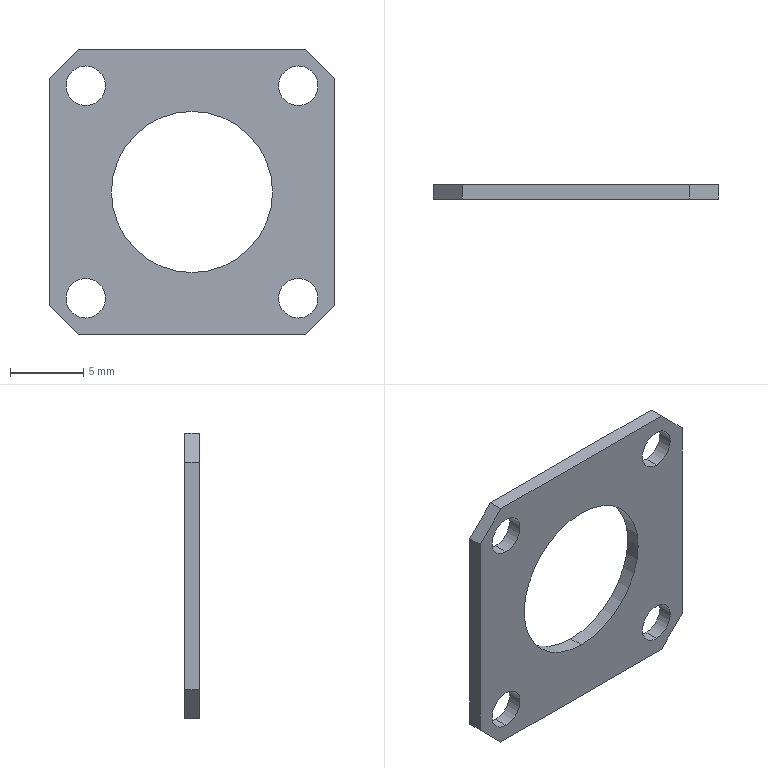Part | SolidWorks | features Extrusion 1, ICE 1 | 1 solid | 20 faces | box 19.5 x 1 x 19.5 mm | volume 254.315 mm3 | cylinder 10 | plane 10 | commonest cylinder face diameters 2.7 x8 11 x2
STEP:
#1=CARTESIAN_POINT('',(-7.25,0.,5.9));
#2=VERTEX_POINT('',#1);
#3=CARTESIAN_POINT('',(-7.25,0.,8.6));
#4=VERTEX_POINT('',#3);
#5=CARTESIAN_POINT('',(-7.25,0.,7.25));
#6=DIRECTION('',(0.,1.,0.));
#7=DIRECTION('',(0.,0.,1.));
#8=AXIS2_PLACEMENT_3D('',#5,#6,#7);
#9=CIRCLE('',#8,1.35);
#10=EDGE_CURVE('',#2,#4,#9,.T.);
#11=ORIENTED_EDGE('',*,*,#10,.F.);
#12=CARTESIAN_POINT('',(-7.25,1.,5.9));
#13=VERTEX_POINT('',#12);
#14=CARTESIAN_POINT('',(-7.25,0.,5.9));
#15=DIRECTION('',(0.,1.,0.));
#16=VECTOR('',#15,1000.);
#17=LINE('',#14,#16);
#18=EDGE_CURVE('',#2,#13,#17,.T.);
#19=ORIENTED_EDGE('',*,*,#18,.T.);
#20=CARTESIAN_POINT('',(-7.25,1.,8.6));
#21=VERTEX_POINT('',#20);
#22=CARTESIAN_POINT('',(-7.25,1.,7.25));
#23=DIRECTION('',(0.,1.,0.));
#24=DIRECTION('',(0.,0.,1.));
#25=AXIS2_PLACEMENT_3D('',#22,#23,#24);
#26=CIRCLE('',#25,1.35);
#27=EDGE_CURVE('',#13,#21,#26,.T.);
#28=ORIENTED_EDGE('',*,*,#27,.T.);
#29=CARTESIAN_POINT('',(-7.25,0.,8.6));
#30=DIRECTION('',(0.,1.,0.));
#31=VECTOR('',#30,1000.);
#32=LINE('',#29,#31);
#33=EDGE_CURVE('',#4,#21,#32,.T.);
#34=ORIENTED_EDGE('',*,*,#33,.F.);
#35=EDGE_LOOP('',(#11,#19,#28,#34));
#36=FACE_OUTER_BOUND('',#35,.T.);
#37=CARTESIAN_POINT('',(-7.25,0.,7.25));
#38=DIRECTION('',(0.,1.,0.));
#39=DIRECTION('',(0.,0.,1.));
#40=AXIS2_PLACEMENT_3D('',#37,#38,#39);
#41=CYLINDRICAL_SURFACE('',#40,1.35);
#42=ADVANCED_FACE('',(#36),#41,.F.);
#43=CARTESIAN_POINT('',(7.25,0.,5.9));
#44=VERTEX_POINT('',#43);
#45=CARTESIAN_POINT('',(7.25,0.,8.6));
#46=VERTEX_POINT('',#45);
#47=CARTESIAN_POINT('',(7.25,0.,7.25));
#48=DIRECTION('',(0.,1.,0.));
#49=DIRECTION('',(0.,0.,1.));
#50=AXIS2_PLACEMENT_3D('',#47,#48,#49);
#51=CIRCLE('',#50,1.35);
#52=EDGE_CURVE('',#44,#46,#51,.T.);
#53=ORIENTED_EDGE('',*,*,#52,.F.);
#54=CARTESIAN_POINT('',(7.25,1.,5.9));
#55=VERTEX_POINT('',#54);
#56=CARTESIAN_POINT('',(7.25,0.,5.9));
#57=DIRECTION('',(0.,1.,0.));
#58=VECTOR('',#57,1000.);
#59=LINE('',#56,#58);
#60=EDGE_CURVE('',#44,#55,#59,.T.);
#61=ORIENTED_EDGE('',*,*,#60,.T.);
#62=CARTESIAN_POINT('',(7.25,1.,8.6));
#63=VERTEX_POINT('',#62);
#64=CARTESIAN_POINT('',(7.25,1.,7.25));
#65=DIRECTION('',(0.,1.,0.));
#66=DIRECTION('',(0.,0.,1.));
#67=AXIS2_PLACEMENT_3D('',#64,#65,#66);
#68=CIRCLE('',#67,1.35);
#69=EDGE_CURVE('',#55,#63,#68,.T.);
#70=ORIENTED_EDGE('',*,*,#69,.T.);
#71=CARTESIAN_POINT('',(7.25,0.,8.6));
#72=DIRECTION('',(0.,1.,0.));
#73=VECTOR('',#72,1000.);
#74=LINE('',#71,#73);
#75=EDGE_CURVE('',#46,#63,#74,.T.);
#76=ORIENTED_EDGE('',*,*,#75,.F.);
#77=EDGE_LOOP('',(#53,#61,#70,#76));
#78=FACE_OUTER_BOUND('',#77,.T.);
#79=CARTESIAN_POINT('',(7.25,0.,7.25));
#80=DIRECTION('',(0.,1.,0.));
#81=DIRECTION('',(0.,0.,1.));
#82=AXIS2_PLACEMENT_3D('',#79,#80,#81);
#83=CYLINDRICAL_SURFACE('',#82,1.35);
#84=ADVANCED_FACE('',(#78),#83,.F.);
#85=CARTESIAN_POINT('',(7.25,0.,-8.6));
#86=VERTEX_POINT('',#85);
#87=CARTESIAN_POINT('',(7.25,0.,-5.9));
#88=VERTEX_POINT('',#87);
#89=CARTESIAN_POINT('',(7.25,0.,-7.25));
#90=DIRECTION('',(0.,1.,0.));
#91=DIRECTION('',(0.,0.,1.));
#92=AXIS2_PLACEMENT_3D('',#89,#90,#91);
#93=CIRCLE('',#92,1.35);
#94=EDGE_CURVE('',#86,#88,#93,.T.);
#95=ORIENTED_EDGE('',*,*,#94,.F.);
#96=CARTESIAN_POINT('',(7.25,1.,-8.6));
#97=VERTEX_POINT('',#96);
#98=CARTESIAN_POINT('',(7.25,0.,-8.6));
#99=DIRECTION('',(0.,1.,0.));
#100=VECTOR('',#99,1000.);
#101=LINE('',#98,#100);
#102=EDGE_CURVE('',#86,#97,#101,.T.);
#103=ORIENTED_EDGE('',*,*,#102,.T.);
#104=CARTESIAN_POINT('',(7.25,1.,-5.9));
#105=VERTEX_POINT('',#104);
#106=CARTESIAN_POINT('',(7.25,1.,-7.25));
#107=DIRECTION('',(0.,1.,0.));
#108=DIRECTION('',(0.,0.,1.));
#109=AXIS2_PLACEMENT_3D('',#106,#107,#108);
#110=CIRCLE('',#109,1.35);
#111=EDGE_CURVE('',#97,#105,#110,.T.);
#112=ORIENTED_EDGE('',*,*,#111,.T.);
#113=CARTESIAN_POINT('',(7.25,0.,-5.9));
#114=DIRECTION('',(0.,1.,0.));
#115=VECTOR('',#114,1000.);
#116=LINE('',#113,#115);
#117=EDGE_CURVE('',#88,#105,#116,.T.);
#118=ORIENTED_EDGE('',*,*,#117,.F.);
#119=EDGE_LOOP('',(#95,#103,#112,#118));
#120=FACE_OUTER_BOUND('',#119,.T.);
#121=CARTESIAN_POINT('',(7.25,0.,-7.25));
#122=DIRECTION('',(0.,1.,0.));
#123=DIRECTION('',(0.,0.,1.));
#124=AXIS2_PLACEMENT_3D('',#121,#122,#123);
#125=CYLINDRICAL_SURFACE('',#124,1.35);
#126=ADVANCED_FACE('',(#120),#125,.F.);
#127=CARTESIAN_POINT('',(-7.25,0.,-8.6));
#128=VERTEX_POINT('',#127);
#129=CARTESIAN_POINT('',(-7.25,0.,-5.9));
#130=VERTEX_POINT('',#129);
#131=CARTESIAN_POINT('',(-7.25,0.,-7.25));
#132=DIRECTION('',(0.,1.,0.));
#133=DIRECTION('',(0.,0.,1.));
#134=AXIS2_PLACEMENT_3D('',#131,#132,#133);
#135=CIRCLE('',#134,1.35);
#136=EDGE_CURVE('',#128,#130,#135,.T.);
#137=ORIENTED_EDGE('',*,*,#136,.F.);
#138=CARTESIAN_POINT('',(-7.25,1.,-8.6));
#139=VERTEX_POINT('',#138);
#140=CARTESIAN_POINT('',(-7.25,0.,-8.6));
#141=DIRECTION('',(0.,1.,0.));
#142=VECTOR('',#141,1000.);
#143=LINE('',#140,#142);
#144=EDGE_CURVE('',#128,#139,#143,.T.);
#145=ORIENTED_EDGE('',*,*,#144,.T.);
#146=CARTESIAN_POINT('',(-7.25,1.,-5.9));
#147=VERTEX_POINT('',#146);
#148=CARTESIAN_POINT('',(-7.25,1.,-7.25));
#149=DIRECTION('',(0.,1.,0.));
#150=DIRECTION('',(0.,0.,1.));
#151=AXIS2_PLACEMENT_3D('',#148,#149,#150);
#152=CIRCLE('',#151,1.35);
#153=EDGE_CURVE('',#139,#147,#152,.T.);
#154=ORIENTED_EDGE('',*,*,#153,.T.);
#155=CARTESIAN_POINT('',(-7.25,0.,-5.9));
#156=DIRECTION('',(0.,1.,0.));
#157=VECTOR('',#156,1000.);
#158=LINE('',#155,#157);
#159=EDGE_CURVE('',#130,#147,#158,.T.);
#160=ORIENTED_EDGE('',*,*,#159,.F.);
#161=EDGE_LOOP('',(#137,#145,#154,#160));
#162=FACE_OUTER_BOUND('',#161,.T.);
#163=CARTESIAN_POINT('',(-7.25,0.,-7.25));
#164=DIRECTION('',(0.,1.,0.));
#165=DIRECTION('',(0.,0.,1.));
#166=AXIS2_PLACEMENT_3D('',#163,#164,#165);
#167=CYLINDRICAL_SURFACE('',#166,1.35);
#168=ADVANCED_FACE('',(#162),#167,.F.);
#169=CARTESIAN_POINT('',(0.,1.,-5.5));
#170=VERTEX_POINT('',#169);
#171=CARTESIAN_POINT('',(0.,1.,5.5));
#172=VERTEX_POINT('',#171);
#173=CARTESIAN_POINT('',(0.,1.,0.));
#174=DIRECTION('',(0.,1.,0.));
#175=DIRECTION('',(0.,0.,1.));
#176=AXIS2_PLACEMENT_3D('',#173,#174,#175);
#177=CIRCLE('',#176,5.5);
#178=EDGE_CURVE('',#170,#172,#177,.T.);
#179=ORIENTED_EDGE('',*,*,#178,.T.);
#180=CARTESIAN_POINT('',(0.,0.,5.5));
#181=VERTEX_POINT('',#180);
#182=CARTESIAN_POINT('',(0.,1.,5.5));
#183=DIRECTION('',(0.,-1.,0.));
#184=VECTOR('',#183,1000.);
#185=LINE('',#182,#184);
#186=EDGE_CURVE('',#172,#181,#185,.T.);
#187=ORIENTED_EDGE('',*,*,#186,.T.);
#188=CARTESIAN_POINT('',(0.,0.,-5.5));
#189=VERTEX_POINT('',#188);
#190=CARTESIAN_POINT('',(0.,0.,0.));
#191=DIRECTION('',(0.,1.,0.));
#192=DIRECTION('',(0.,0.,1.));
#193=AXIS2_PLACEMENT_3D('',#190,#191,#192);
#194=CIRCLE('',#193,5.5);
#195=EDGE_CURVE('',#189,#181,#194,.T.);
#196=ORIENTED_EDGE('',*,*,#195,.F.);
#197=CARTESIAN_POINT('',(0.,1.,-5.5));
#198=DIRECTION('',(0.,-1.,0.));
#199=VECTOR('',#198,1000.);
#200=LINE('',#197,#199);
#201=EDGE_CURVE('',#170,#189,#200,.T.);
#202=ORIENTED_EDGE('',*,*,#201,.F.);
#203=EDGE_LOOP('',(#179,#187,#196,#202));
#204=FACE_OUTER_BOUND('',#203,.T.);
#205=CARTESIAN_POINT('',(0.,1.,0.));
#206=DIRECTION('',(0.,-1.,0.));
#207=DIRECTION('',(0.,0.,-1.));
#208=AXIS2_PLACEMENT_3D('',#205,#206,#207);
#209=CYLINDRICAL_SURFACE('',#208,5.5);
#210=ADVANCED_FACE('',(#204),#209,.F.);
#211=CARTESIAN_POINT('',(-7.25,1.,7.25));
#212=DIRECTION('',(0.,1.,0.));
#213=DIRECTION('',(0.,0.,1.));
#214=AXIS2_PLACEMENT_3D('',#211,#212,#213);
#215=CIRCLE('',#214,1.35);
#216=EDGE_CURVE('',#21,#13,#215,.T.);
#217=ORIENTED_EDGE('',*,*,#216,.F.);
#218=ORIENTED_EDGE('',*,*,#27,.F.);
#219=EDGE_LOOP('',(#217,#218));
#220=FACE_BOUND('',#219,.T.);
#221=CARTESIAN_POINT('',(7.25,1.,7.25));
#222=DIRECTION('',(0.,1.,0.));
#223=DIRECTION('',(0.,0.,1.));
#224=AXIS2_PLACEMENT_3D('',#221,#222,#223);
#225=CIRCLE('',#224,1.35);
#226=EDGE_CURVE('',#63,#55,#225,.T.);
#227=ORIENTED_EDGE('',*,*,#226,.F.);
#228=ORIENTED_EDGE('',*,*,#69,.F.);
#229=EDGE_LOOP('',(#227,#228));
#230=FACE_BOUND('',#229,.T.);
#231=CARTESIAN_POINT('',(7.25,1.,-7.25));
#232=DIRECTION('',(0.,1.,0.));
#233=DIRECTION('',(0.,0.,1.));
#234=AXIS2_PLACEMENT_3D('',#231,#232,#233);
#235=CIRCLE('',#234,1.35);
#236=EDGE_CURVE('',#105,#97,#235,.T.);
#237=ORIENTED_EDGE('',*,*,#236,.F.);
#238=ORIENTED_EDGE('',*,*,#111,.F.);
#239=EDGE_LOOP('',(#237,#238));
#240=FACE_BOUND('',#239,.T.);
#241=CARTESIAN_POINT('',(-7.25,1.,-7.25));
#242=DIRECTION('',(0.,1.,0.));
#243=DIRECTION('',(0.,0.,1.));
#244=AXIS2_PLACEMENT_3D('',#241,#242,#243);
#245=CIRCLE('',#244,1.35);
#246=EDGE_CURVE('',#147,#139,#245,.T.);
#247=ORIENTED_EDGE('',*,*,#246,.F.);
#248=ORIENTED_EDGE('',*,*,#153,.F.);
#249=EDGE_LOOP('',(#247,#248));
#250=FACE_BOUND('',#249,.T.);
#251=CARTESIAN_POINT('',(-7.75,1.,9.75));
#252=VERTEX_POINT('',#251);
#253=CARTESIAN_POINT('',(7.75,1.,9.75));
#254=VERTEX_POINT('',#253);
#255=CARTESIAN_POINT('',(-7.75,1.,9.75));
#256=DIRECTION('',(1.,0.,0.));
#257=VECTOR('',#256,1000.);
#258=LINE('',#255,#257);
#259=EDGE_CURVE('',#252,#254,#258,.T.);
#260=ORIENTED_EDGE('',*,*,#259,.T.);
#261=CARTESIAN_POINT('',(9.75,1.,7.75));
#262=VERTEX_POINT('',#261);
#263=CARTESIAN_POINT('',(7.75,1.,9.75));
#264=DIRECTION('',(0.7071,0.,-0.7071));
#265=VECTOR('',#264,1000.);
#266=LINE('',#263,#265);
#267=EDGE_CURVE('',#254,#262,#266,.T.);
#268=ORIENTED_EDGE('',*,*,#267,.T.);
#269=CARTESIAN_POINT('',(9.75,1.,-7.75));
#270=VERTEX_POINT('',#269);
#271=CARTESIAN_POINT('',(9.75,1.,-7.75));
#272=DIRECTION('',(0.,0.,-1.));
#273=VECTOR('',#272,1000.);
#274=LINE('',#271,#273);
#275=EDGE_CURVE('',#262,#270,#274,.T.);
#276=ORIENTED_EDGE('',*,*,#275,.T.);
#277=CARTESIAN_POINT('',(7.75,1.,-9.75));
#278=VERTEX_POINT('',#277);
#279=CARTESIAN_POINT('',(7.75,1.,-9.75));
#280=DIRECTION('',(-0.7071,0.,-0.7071));
#281=VECTOR('',#280,1000.);
#282=LINE('',#279,#281);
#283=EDGE_CURVE('',#270,#278,#282,.T.);
#284=ORIENTED_EDGE('',*,*,#283,.T.);
#285=CARTESIAN_POINT('',(-7.75,1.,-9.75));
#286=VERTEX_POINT('',#285);
#287=CARTESIAN_POINT('',(-7.75,1.,-9.75));
#288=DIRECTION('',(-1.,0.,0.));
#289=VECTOR('',#288,1000.);
#290=LINE('',#287,#289);
#291=EDGE_CURVE('',#278,#286,#290,.T.);
#292=ORIENTED_EDGE('',*,*,#291,.T.);
#293=CARTESIAN_POINT('',(-9.75,1.,-7.75));
#294=VERTEX_POINT('',#293);
#295=CARTESIAN_POINT('',(-9.75,1.,-7.75));
#296=DIRECTION('',(-0.7071,0.,0.7071));
#297=VECTOR('',#296,1000.);
#298=LINE('',#295,#297);
#299=EDGE_CURVE('',#286,#294,#298,.T.);
#300=ORIENTED_EDGE('',*,*,#299,.T.);
#301=CARTESIAN_POINT('',(-9.75,1.,7.75));
#302=VERTEX_POINT('',#301);
#303=CARTESIAN_POINT('',(-9.75,1.,-7.75));
#304=DIRECTION('',(0.,0.,1.));
#305=VECTOR('',#304,1000.);
#306=LINE('',#303,#305);
#307=EDGE_CURVE('',#294,#302,#306,.T.);
#308=ORIENTED_EDGE('',*,*,#307,.T.);
#309=CARTESIAN_POINT('',(-9.75,1.,7.75));
#310=DIRECTION('',(0.7071,0.,0.7071));
#311=VECTOR('',#310,1000.);
#312=LINE('',#309,#311);
#313=EDGE_CURVE('',#302,#252,#312,.T.);
#314=ORIENTED_EDGE('',*,*,#313,.T.);
#315=EDGE_LOOP('',(#260,#268,#276,#284,#292,#300,#308,#314));
#316=FACE_OUTER_BOUND('',#315,.T.);
#317=ORIENTED_EDGE('',*,*,#178,.F.);
#318=CARTESIAN_POINT('',(0.,1.,0.));
#319=DIRECTION('',(0.,1.,0.));
#320=DIRECTION('',(0.,0.,1.));
#321=AXIS2_PLACEMENT_3D('',#318,#319,#320);
#322=CIRCLE('',#321,5.5);
#323=EDGE_CURVE('',#172,#170,#322,.T.);
#324=ORIENTED_EDGE('',*,*,#323,.F.);
#325=EDGE_LOOP('',(#317,#324));
#326=FACE_BOUND('',#325,.T.);
#327=CARTESIAN_POINT('',(0.,1.,0.));
#328=DIRECTION('',(0.,-1.,0.));
#329=DIRECTION('',(0.,0.,-1.));
#330=AXIS2_PLACEMENT_3D('',#327,#328,#329);
#331=PLANE('',#330);
#332=ADVANCED_FACE('',(#220,#230,#240,#250,#316,#326),#331,.F.);
#333=CARTESIAN_POINT('',(-7.25,0.,7.25));
#334=DIRECTION('',(0.,1.,0.));
#335=DIRECTION('',(0.,0.,1.));
#336=AXIS2_PLACEMENT_3D('',#333,#334,#335);
#337=CIRCLE('',#336,1.35);
#338=EDGE_CURVE('',#4,#2,#337,.T.);
#339=ORIENTED_EDGE('',*,*,#338,.T.);
#340=ORIENTED_EDGE('',*,*,#10,.T.);
#341=EDGE_LOOP('',(#339,#340));
#342=FACE_BOUND('',#341,.T.);
#343=CARTESIAN_POINT('',(7.25,0.,7.25));
#344=DIRECTION('',(0.,1.,0.));
#345=DIRECTION('',(0.,0.,1.));
#346=AXIS2_PLACEMENT_3D('',#343,#344,#345);
#347=CIRCLE('',#346,1.35);
#348=EDGE_CURVE('',#46,#44,#347,.T.);
#349=ORIENTED_EDGE('',*,*,#348,.T.);
#350=ORIENTED_EDGE('',*,*,#52,.T.);
#351=EDGE_LOOP('',(#349,#350));
#352=FACE_BOUND('',#351,.T.);
#353=CARTESIAN_POINT('',(7.25,0.,-7.25));
#354=DIRECTION('',(0.,1.,0.));
#355=DIRECTION('',(0.,0.,1.));
#356=AXIS2_PLACEMENT_3D('',#353,#354,#355);
#357=CIRCLE('',#356,1.35);
#358=EDGE_CURVE('',#88,#86,#357,.T.);
#359=ORIENTED_EDGE('',*,*,#358,.T.);
#360=ORIENTED_EDGE('',*,*,#94,.T.);
#361=EDGE_LOOP('',(#359,#360));
#362=FACE_BOUND('',#361,.T.);
#363=CARTESIAN_POINT('',(-7.25,0.,-7.25));
#364=DIRECTION('',(0.,1.,0.));
#365=DIRECTION('',(0.,0.,1.));
#366=AXIS2_PLACEMENT_3D('',#363,#364,#365);
#367=CIRCLE('',#366,1.35);
#368=EDGE_CURVE('',#130,#128,#367,.T.);
#369=ORIENTED_EDGE('',*,*,#368,.T.);
#370=ORIENTED_EDGE('',*,*,#136,.T.);
#371=EDGE_LOOP('',(#369,#370));
#372=FACE_BOUND('',#371,.T.);
#373=CARTESIAN_POINT('',(-7.75,0.,9.75));
#374=VERTEX_POINT('',#373);
#375=CARTESIAN_POINT('',(7.75,0.,9.75));
#376=VERTEX_POINT('',#375);
#377=CARTESIAN_POINT('',(-7.75,0.,9.75));
#378=DIRECTION('',(1.,0.,0.));
#379=VECTOR('',#378,1000.);
#380=LINE('',#377,#379);
#381=EDGE_CURVE('',#374,#376,#380,.T.);
#382=ORIENTED_EDGE('',*,*,#381,.F.);
#383=CARTESIAN_POINT('',(-9.75,0.,7.75));
#384=VERTEX_POINT('',#383);
#385=CARTESIAN_POINT('',(-9.75,0.,7.75));
#386=DIRECTION('',(0.7071,0.,0.7071));
#387=VECTOR('',#386,1000.);
#388=LINE('',#385,#387);
#389=EDGE_CURVE('',#384,#374,#388,.T.);
#390=ORIENTED_EDGE('',*,*,#389,.F.);
#391=CARTESIAN_POINT('',(-9.75,0.,-7.75));
#392=VERTEX_POINT('',#391);
#393=CARTESIAN_POINT('',(-9.75,0.,-7.75));
#394=DIRECTION('',(0.,0.,1.));
#395=VECTOR('',#394,1000.);
#396=LINE('',#393,#395);
#397=EDGE_CURVE('',#392,#384,#396,.T.);
#398=ORIENTED_EDGE('',*,*,#397,.F.);
#399=CARTESIAN_POINT('',(-7.75,0.,-9.75));
#400=VERTEX_POINT('',#399);
#401=CARTESIAN_POINT('',(-9.75,0.,-7.75));
#402=DIRECTION('',(-0.7071,0.,0.7071));
#403=VECTOR('',#402,1000.);
#404=LINE('',#401,#403);
#405=EDGE_CURVE('',#400,#392,#404,.T.);
#406=ORIENTED_EDGE('',*,*,#405,.F.);
#407=CARTESIAN_POINT('',(7.75,0.,-9.75));
#408=VERTEX_POINT('',#407);
#409=CARTESIAN_POINT('',(-7.75,0.,-9.75));
#410=DIRECTION('',(-1.,0.,0.));
#411=VECTOR('',#410,1000.);
#412=LINE('',#409,#411);
#413=EDGE_CURVE('',#408,#400,#412,.T.);
#414=ORIENTED_EDGE('',*,*,#413,.F.);
#415=CARTESIAN_POINT('',(9.75,0.,-7.75));
#416=VERTEX_POINT('',#415);
#417=CARTESIAN_POINT('',(7.75,0.,-9.75));
#418=DIRECTION('',(-0.7071,0.,-0.7071));
#419=VECTOR('',#418,1000.);
#420=LINE('',#417,#419);
#421=EDGE_CURVE('',#416,#408,#420,.T.);
#422=ORIENTED_EDGE('',*,*,#421,.F.);
#423=CARTESIAN_POINT('',(9.75,0.,7.75));
#424=VERTEX_POINT('',#423);
#425=CARTESIAN_POINT('',(9.75,0.,-7.75));
#426=DIRECTION('',(0.,0.,-1.));
#427=VECTOR('',#426,1000.);
#428=LINE('',#425,#427);
#429=EDGE_CURVE('',#424,#416,#428,.T.);
#430=ORIENTED_EDGE('',*,*,#429,.F.);
#431=CARTESIAN_POINT('',(7.75,0.,9.75));
#432=DIRECTION('',(0.7071,0.,-0.7071));
#433=VECTOR('',#432,1000.);
#434=LINE('',#431,#433);
#435=EDGE_CURVE('',#376,#424,#434,.T.);
#436=ORIENTED_EDGE('',*,*,#435,.F.);
#437=EDGE_LOOP('',(#382,#390,#398,#406,#414,#422,#430,#436));
#438=FACE_OUTER_BOUND('',#437,.T.);
#439=ORIENTED_EDGE('',*,*,#195,.T.);
#440=CARTESIAN_POINT('',(0.,0.,0.));
#441=DIRECTION('',(0.,1.,0.));
#442=DIRECTION('',(0.,0.,1.));
#443=AXIS2_PLACEMENT_3D('',#440,#441,#442);
#444=CIRCLE('',#443,5.5);
#445=EDGE_CURVE('',#181,#189,#444,.T.);
#446=ORIENTED_EDGE('',*,*,#445,.T.);
#447=EDGE_LOOP('',(#439,#446));
#448=FACE_BOUND('',#447,.T.);
#449=CARTESIAN_POINT('',(0.,0.,0.));
#450=DIRECTION('',(0.,-1.,0.));
#451=DIRECTION('',(0.,0.,-1.));
#452=AXIS2_PLACEMENT_3D('',#449,#450,#451);
#453=PLANE('',#452);
#454=ADVANCED_FACE('',(#342,#352,#362,#372,#438,#448),#453,.T.);
#455=ORIENTED_EDGE('',*,*,#381,.T.);
#456=CARTESIAN_POINT('',(7.75,1.,9.75));
#457=DIRECTION('',(0.,-1.,0.));
#458=VECTOR('',#457,1000.);
#459=LINE('',#456,#458);
#460=EDGE_CURVE('',#254,#376,#459,.T.);
#461=ORIENTED_EDGE('',*,*,#460,.F.);
#462=ORIENTED_EDGE('',*,*,#259,.F.);
#463=CARTESIAN_POINT('',(-7.75,1.,9.75));
#464=DIRECTION('',(0.,-1.,0.));
#465=VECTOR('',#464,1000.);
#466=LINE('',#463,#465);
#467=EDGE_CURVE('',#252,#374,#466,.T.);
#468=ORIENTED_EDGE('',*,*,#467,.T.);
#469=EDGE_LOOP('',(#455,#461,#462,#468));
#470=FACE_OUTER_BOUND('',#469,.T.);
#471=CARTESIAN_POINT('',(-7.75,1.,9.75));
#472=DIRECTION('',(0.,0.,-1.));
#473=DIRECTION('',(-1.,0.,0.));
#474=AXIS2_PLACEMENT_3D('',#471,#472,#473);
#475=PLANE('',#474);
#476=ADVANCED_FACE('',(#470),#475,.F.);
#477=ORIENTED_EDGE('',*,*,#435,.T.);
#478=CARTESIAN_POINT('',(9.75,1.,7.75));
#479=DIRECTION('',(0.,-1.,0.));
#480=VECTOR('',#479,1000.);
#481=LINE('',#478,#480);
#482=EDGE_CURVE('',#262,#424,#481,.T.);
#483=ORIENTED_EDGE('',*,*,#482,.F.);
#484=ORIENTED_EDGE('',*,*,#267,.F.);
#485=ORIENTED_EDGE('',*,*,#460,.T.);
#486=EDGE_LOOP('',(#477,#483,#484,#485));
#487=FACE_OUTER_BOUND('',#486,.T.);
#488=CARTESIAN_POINT('',(7.75,1.,9.75));
#489=DIRECTION('',(-0.7071,0.,-0.7071));
#490=DIRECTION('',(-0.7071,0.,0.7071));
#491=AXIS2_PLACEMENT_3D('',#488,#489,#490);
#492=PLANE('',#491);
#493=ADVANCED_FACE('',(#487),#492,.F.);
#494=ORIENTED_EDGE('',*,*,#429,.T.);
#495=CARTESIAN_POINT('',(9.75,1.,-7.75));
#496=DIRECTION('',(0.,-1.,0.));
#497=VECTOR('',#496,1000.);
#498=LINE('',#495,#497);
#499=EDGE_CURVE('',#270,#416,#498,.T.);
#500=ORIENTED_EDGE('',*,*,#499,.F.);
#501=ORIENTED_EDGE('',*,*,#275,.F.);
#502=ORIENTED_EDGE('',*,*,#482,.T.);
#503=EDGE_LOOP('',(#494,#500,#501,#502));
#504=FACE_OUTER_BOUND('',#503,.T.);
#505=CARTESIAN_POINT('',(9.75,1.,-7.75));
#506=DIRECTION('',(-1.,0.,0.));
#507=DIRECTION('',(0.,0.,1.));
#508=AXIS2_PLACEMENT_3D('',#505,#506,#507);
#509=PLANE('',#508);
#510=ADVANCED_FACE('',(#504),#509,.F.);
#511=ORIENTED_EDGE('',*,*,#421,.T.);
#512=CARTESIAN_POINT('',(7.75,1.,-9.75));
#513=DIRECTION('',(0.,-1.,0.));
#514=VECTOR('',#513,1000.);
#515=LINE('',#512,#514);
#516=EDGE_CURVE('',#278,#408,#515,.T.);
#517=ORIENTED_EDGE('',*,*,#516,.F.);
#518=ORIENTED_EDGE('',*,*,#283,.F.);
#519=ORIENTED_EDGE('',*,*,#499,.T.);
#520=EDGE_LOOP('',(#511,#517,#518,#519));
#521=FACE_OUTER_BOUND('',#520,.T.);
#522=CARTESIAN_POINT('',(7.75,1.,-9.75));
#523=DIRECTION('',(-0.7071,0.,0.7071));
#524=DIRECTION('',(0.7071,0.,0.7071));
#525=AXIS2_PLACEMENT_3D('',#522,#523,#524);
#526=PLANE('',#525);
#527=ADVANCED_FACE('',(#521),#526,.F.);
#528=ORIENTED_EDGE('',*,*,#413,.T.);
#529=CARTESIAN_POINT('',(-7.75,1.,-9.75));
#530=DIRECTION('',(0.,-1.,0.));
#531=VECTOR('',#530,1000.);
#532=LINE('',#529,#531);
#533=EDGE_CURVE('',#286,#400,#532,.T.);
#534=ORIENTED_EDGE('',*,*,#533,.F.);
#535=ORIENTED_EDGE('',*,*,#291,.F.);
#536=ORIENTED_EDGE('',*,*,#516,.T.);
#537=EDGE_LOOP('',(#528,#534,#535,#536));
#538=FACE_OUTER_BOUND('',#537,.T.);
#539=CARTESIAN_POINT('',(-7.75,1.,-9.75));
#540=DIRECTION('',(0.,0.,1.));
#541=DIRECTION('',(1.,0.,0.));
#542=AXIS2_PLACEMENT_3D('',#539,#540,#541);
#543=PLANE('',#542);
#544=ADVANCED_FACE('',(#538),#543,.F.);
#545=ORIENTED_EDGE('',*,*,#405,.T.);
#546=CARTESIAN_POINT('',(-9.75,1.,-7.75));
#547=DIRECTION('',(0.,-1.,0.));
#548=VECTOR('',#547,1000.);
#549=LINE('',#546,#548);
#550=EDGE_CURVE('',#294,#392,#549,.T.);
#551=ORIENTED_EDGE('',*,*,#550,.F.);
#552=ORIENTED_EDGE('',*,*,#299,.F.);
#553=ORIENTED_EDGE('',*,*,#533,.T.);
#554=EDGE_LOOP('',(#545,#551,#552,#553));
#555=FACE_OUTER_BOUND('',#554,.T.);
#556=CARTESIAN_POINT('',(-9.75,1.,-7.75));
#557=DIRECTION('',(0.7071,0.,0.7071));
#558=DIRECTION('',(0.7071,0.,-0.7071));
#559=AXIS2_PLACEMENT_3D('',#556,#557,#558);
#560=PLANE('',#559);
#561=ADVANCED_FACE('',(#555),#560,.F.);
#562=ORIENTED_EDGE('',*,*,#397,.T.);
#563=CARTESIAN_POINT('',(-9.75,1.,7.75));
#564=DIRECTION('',(0.,-1.,0.));
#565=VECTOR('',#564,1000.);
#566=LINE('',#563,#565);
#567=EDGE_CURVE('',#302,#384,#566,.T.);
#568=ORIENTED_EDGE('',*,*,#567,.F.);
#569=ORIENTED_EDGE('',*,*,#307,.F.);
#570=ORIENTED_EDGE('',*,*,#550,.T.);
#571=EDGE_LOOP('',(#562,#568,#569,#570));
#572=FACE_OUTER_BOUND('',#571,.T.);
#573=CARTESIAN_POINT('',(-9.75,1.,-7.75));
#574=DIRECTION('',(1.,0.,0.));
#575=DIRECTION('',(0.,0.,-1.));
#576=AXIS2_PLACEMENT_3D('',#573,#574,#575);
#577=PLANE('',#576);
#578=ADVANCED_FACE('',(#572),#577,.F.);
#579=ORIENTED_EDGE('',*,*,#389,.T.);
#580=ORIENTED_EDGE('',*,*,#467,.F.);
#581=ORIENTED_EDGE('',*,*,#313,.F.);
#582=ORIENTED_EDGE('',*,*,#567,.T.);
#583=EDGE_LOOP('',(#579,#580,#581,#582));
#584=FACE_OUTER_BOUND('',#583,.T.);
#585=CARTESIAN_POINT('',(-9.75,1.,7.75));
#586=DIRECTION('',(0.7071,0.,-0.7071));
#587=DIRECTION('',(-0.7071,0.,-0.7071));
#588=AXIS2_PLACEMENT_3D('',#585,#586,#587);
#589=PLANE('',#588);
#590=ADVANCED_FACE('',(#584),#589,.F.);
#591=ORIENTED_EDGE('',*,*,#186,.F.);
#592=ORIENTED_EDGE('',*,*,#323,.T.);
#593=ORIENTED_EDGE('',*,*,#201,.T.);
#594=ORIENTED_EDGE('',*,*,#445,.F.);
#595=EDGE_LOOP('',(#591,#592,#593,#594));
#596=FACE_OUTER_BOUND('',#595,.T.);
#597=CARTESIAN_POINT('',(0.,1.,0.));
#598=DIRECTION('',(0.,-1.,0.));
#599=DIRECTION('',(0.,0.,-1.));
#600=AXIS2_PLACEMENT_3D('',#597,#598,#599);
#601=CYLINDRICAL_SURFACE('',#600,5.5);
#602=ADVANCED_FACE('',(#596),#601,.F.);
#603=ORIENTED_EDGE('',*,*,#144,.F.);
#604=ORIENTED_EDGE('',*,*,#368,.F.);
#605=ORIENTED_EDGE('',*,*,#159,.T.);
#606=ORIENTED_EDGE('',*,*,#246,.T.);
#607=EDGE_LOOP('',(#603,#604,#605,#606));
#608=FACE_OUTER_BOUND('',#607,.T.);
#609=CARTESIAN_POINT('',(-7.25,0.,-7.25));
#610=DIRECTION('',(0.,1.,0.));
#611=DIRECTION('',(0.,0.,1.));
#612=AXIS2_PLACEMENT_3D('',#609,#610,#611);
#613=CYLINDRICAL_SURFACE('',#612,1.35);
#614=ADVANCED_FACE('',(#608),#613,.F.);
#615=ORIENTED_EDGE('',*,*,#102,.F.);
#616=ORIENTED_EDGE('',*,*,#358,.F.);
#617=ORIENTED_EDGE('',*,*,#117,.T.);
#618=ORIENTED_EDGE('',*,*,#236,.T.);
#619=EDGE_LOOP('',(#615,#616,#617,#618));
#620=FACE_OUTER_BOUND('',#619,.T.);
#621=CARTESIAN_POINT('',(7.25,0.,-7.25));
#622=DIRECTION('',(0.,1.,0.));
#623=DIRECTION('',(0.,0.,1.));
#624=AXIS2_PLACEMENT_3D('',#621,#622,#623);
#625=CYLINDRICAL_SURFACE('',#624,1.35);
#626=ADVANCED_FACE('',(#620),#625,.F.);
#627=ORIENTED_EDGE('',*,*,#60,.F.);
#628=ORIENTED_EDGE('',*,*,#348,.F.);
#629=ORIENTED_EDGE('',*,*,#75,.T.);
#630=ORIENTED_EDGE('',*,*,#226,.T.);
#631=EDGE_LOOP('',(#627,#628,#629,#630));
#632=FACE_OUTER_BOUND('',#631,.T.);
#633=CARTESIAN_POINT('',(7.25,0.,7.25));
#634=DIRECTION('',(0.,1.,0.));
#635=DIRECTION('',(0.,0.,1.));
#636=AXIS2_PLACEMENT_3D('',#633,#634,#635);
#637=CYLINDRICAL_SURFACE('',#636,1.35);
#638=ADVANCED_FACE('',(#632),#637,.F.);
#639=ORIENTED_EDGE('',*,*,#18,.F.);
#640=ORIENTED_EDGE('',*,*,#338,.F.);
#641=ORIENTED_EDGE('',*,*,#33,.T.);
#642=ORIENTED_EDGE('',*,*,#216,.T.);
#643=EDGE_LOOP('',(#639,#640,#641,#642));
#644=FACE_OUTER_BOUND('',#643,.T.);
#645=CARTESIAN_POINT('',(-7.25,0.,7.25));
#646=DIRECTION('',(0.,1.,0.));
#647=DIRECTION('',(0.,0.,1.));
#648=AXIS2_PLACEMENT_3D('',#645,#646,#647);
#649=CYLINDRICAL_SURFACE('',#648,1.35);
#650=ADVANCED_FACE('',(#644),#649,.F.);
#651=CLOSED_SHELL('',(#42,#84,#126,#168,#210,#332,#454,#476,#493,#510,#527,#544,#561,#578,#590,#602,#614,#626,#638,#650));
#652=MANIFOLD_SOLID_BREP('',#651);
#653=CARTESIAN_POINT('',(0.,0.,0.));
#654=DIRECTION('',(0.,0.,1.));
#655=DIRECTION('',(1.,0.,0.));
#656=AXIS2_PLACEMENT_3D('',#653,#654,#655);
#657=(LENGTH_UNIT()NAMED_UNIT(*)SI_UNIT(.MILLI.,.METRE.));
#658=UNCERTAINTY_MEASURE_WITH_UNIT(LENGTH_MEASURE(0.00001),#657,'','');
#659=(NAMED_UNIT(*)PLANE_ANGLE_UNIT()SI_UNIT($,.RADIAN.));
#660=(NAMED_UNIT(*)SI_UNIT($,.STERADIAN.)SOLID_ANGLE_UNIT());
#661=(GEOMETRIC_REPRESENTATION_CONTEXT(3)GLOBAL_UNCERTAINTY_ASSIGNED_CONTEXT((#658))GLOBAL_UNIT_ASSIGNED_CONTEXT((#657,#659,#660))REPRESENTATION_CONTEXT('',''));
#662=ADVANCED_BREP_SHAPE_REPRESENTATION('',(#652,#656),#661);